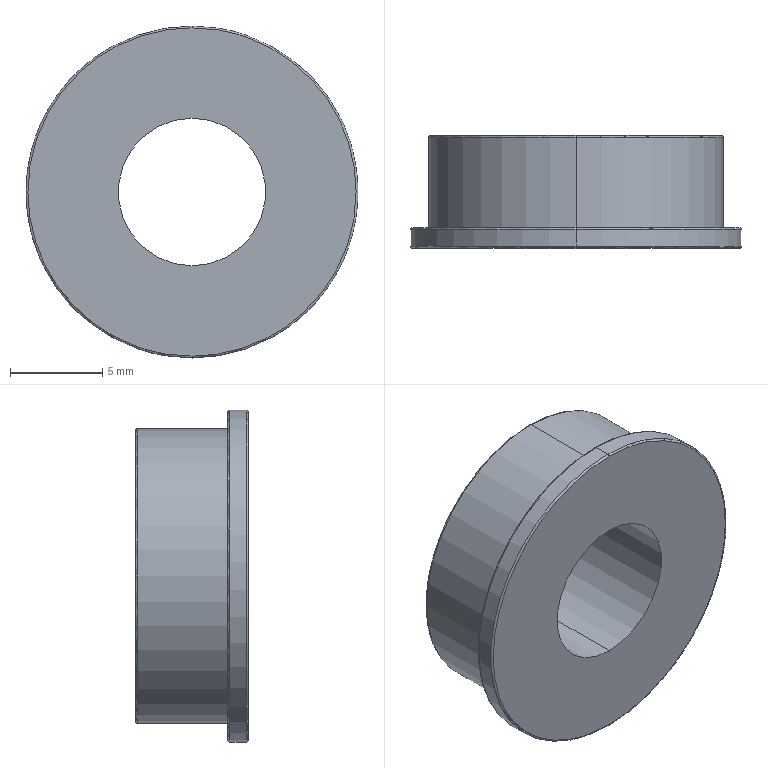Part | NX | features BREP 1 | 1 solid | 15 faces | box 18 x 6.1 x 18 mm | volume 978.51 mm3 | torus 6 | cylinder 6 | plane 3 | commonest cylinder face diameters 8 x2 16 x2 18 x2
STEP:
#1=CARTESIAN_POINT('',(0.,0.,8.9));
#2=VERTEX_POINT('',#1);
#3=CARTESIAN_POINT('',(0.,0.,-8.9));
#4=VERTEX_POINT('',#3);
#5=CARTESIAN_POINT('',(0.,0.,8.9));
#6=CARTESIAN_POINT('',(-0.2723,0.,8.9));
#7=CARTESIAN_POINT('',(-0.6789,0.,8.881));
#8=CARTESIAN_POINT('',(-1.15,0.,8.827));
#9=CARTESIAN_POINT('',(-1.385,0.,8.792));
#10=CARTESIAN_POINT('',(-1.486,0.,8.775));
#11=CARTESIAN_POINT('',(-1.553,0.,8.764));
#12=CARTESIAN_POINT('',(-1.584,0.,8.758));
#13=CARTESIAN_POINT('',(-1.903,0.,8.699));
#14=CARTESIAN_POINT('',(-2.323,0.,8.6));
#15=CARTESIAN_POINT('',(-2.803,0.,8.449));
#16=CARTESIAN_POINT('',(-3.04,0.,8.365));
#17=CARTESIAN_POINT('',(-3.141,0.,8.327));
#18=CARTESIAN_POINT('',(-3.209,0.,8.301));
#19=CARTESIAN_POINT('',(-3.241,0.,8.289));
#20=CARTESIAN_POINT('',(-3.556,0.,8.164));
#21=CARTESIAN_POINT('',(-3.964,0.,7.978));
#22=CARTESIAN_POINT('',(-4.423,0.,7.726));
#23=CARTESIAN_POINT('',(-4.616,0.,7.61));
#24=CARTESIAN_POINT('',(-4.744,0.,7.531));
#25=CARTESIAN_POINT('',(-4.806,0.,7.491));
#26=CARTESIAN_POINT('',(-5.384,0.,7.113));
#27=CARTESIAN_POINT('',(-5.859,0.,6.727));
#28=CARTESIAN_POINT('',(-6.51,0.,6.076));
#29=CARTESIAN_POINT('',(-6.818,0.,5.735));
#30=CARTESIAN_POINT('',(-7.144,0.,5.312));
#31=CARTESIAN_POINT('',(-7.277,0.,5.124));
#32=CARTESIAN_POINT('',(-7.364,0.,4.998));
#33=CARTESIAN_POINT('',(-7.408,0.,4.933));
#34=CARTESIAN_POINT('',(-7.614,0.,4.619));
#35=CARTESIAN_POINT('',(-7.84,0.,4.231));
#36=CARTESIAN_POINT('',(-8.069,0.,3.76));
#37=CARTESIAN_POINT('',(-8.175,0.,3.519));
#38=CARTESIAN_POINT('',(-8.219,0.,3.415));
#39=CARTESIAN_POINT('',(-8.247,0.,3.346));
#40=CARTESIAN_POINT('',(-8.262,0.,3.31));
#41=CARTESIAN_POINT('',(-8.381,0.,3.008));
#42=CARTESIAN_POINT('',(-8.52,0.,2.6));
#43=CARTESIAN_POINT('',(-8.648,0.,2.113));
#44=CARTESIAN_POINT('',(-8.702,0.,1.867));
#45=CARTESIAN_POINT('',(-8.724,0.,1.761));
#46=CARTESIAN_POINT('',(-8.738,0.,1.69));
#47=CARTESIAN_POINT('',(-8.745,0.,1.653));
#48=CARTESIAN_POINT('',(-8.85,0.,1.085));
#49=CARTESIAN_POINT('',(-8.9,0.,0.544));
#50=CARTESIAN_POINT('',(-8.9,0.,-0.272));
#51=CARTESIAN_POINT('',(-8.881,0.,-0.6784));
#52=CARTESIAN_POINT('',(-8.827,0.,-1.15));
#53=CARTESIAN_POINT('',(-8.792,0.,-1.385));
#54=CARTESIAN_POINT('',(-8.775,0.,-1.485));
#55=CARTESIAN_POINT('',(-8.764,0.,-1.553));
#56=CARTESIAN_POINT('',(-8.758,0.,-1.584));
#57=CARTESIAN_POINT('',(-8.699,0.,-1.903));
#58=CARTESIAN_POINT('',(-8.6,0.,-2.323));
#59=CARTESIAN_POINT('',(-8.449,0.,-2.803));
#60=CARTESIAN_POINT('',(-8.365,0.,-3.04));
#61=CARTESIAN_POINT('',(-8.327,0.,-3.141));
#62=CARTESIAN_POINT('',(-8.301,0.,-3.209));
#63=CARTESIAN_POINT('',(-8.289,0.,-3.241));
#64=CARTESIAN_POINT('',(-8.164,0.,-3.556));
#65=CARTESIAN_POINT('',(-7.978,0.,-3.964));
#66=CARTESIAN_POINT('',(-7.726,0.,-4.423));
#67=CARTESIAN_POINT('',(-7.61,0.,-4.616));
#68=CARTESIAN_POINT('',(-7.531,0.,-4.744));
#69=CARTESIAN_POINT('',(-7.491,0.,-4.806));
#70=CARTESIAN_POINT('',(-7.113,0.,-5.384));
#71=CARTESIAN_POINT('',(-6.727,0.,-5.859));
#72=CARTESIAN_POINT('',(-6.076,0.,-6.51));
#73=CARTESIAN_POINT('',(-5.735,0.,-6.818));
#74=CARTESIAN_POINT('',(-5.312,0.,-7.144));
#75=CARTESIAN_POINT('',(-5.124,0.,-7.277));
#76=CARTESIAN_POINT('',(-4.998,0.,-7.364));
#77=CARTESIAN_POINT('',(-4.933,0.,-7.408));
#78=CARTESIAN_POINT('',(-4.619,0.,-7.614));
#79=CARTESIAN_POINT('',(-4.231,0.,-7.84));
#80=CARTESIAN_POINT('',(-3.76,0.,-8.069));
#81=CARTESIAN_POINT('',(-3.519,0.,-8.175));
#82=CARTESIAN_POINT('',(-3.415,0.,-8.219));
#83=CARTESIAN_POINT('',(-3.346,0.,-8.247));
#84=CARTESIAN_POINT('',(-3.31,0.,-8.262));
#85=CARTESIAN_POINT('',(-3.008,0.,-8.381));
#86=CARTESIAN_POINT('',(-2.6,0.,-8.52));
#87=CARTESIAN_POINT('',(-2.113,0.,-8.648));
#88=CARTESIAN_POINT('',(-1.867,0.,-8.702));
#89=CARTESIAN_POINT('',(-1.761,0.,-8.724));
#90=CARTESIAN_POINT('',(-1.69,0.,-8.738));
#91=CARTESIAN_POINT('',(-1.653,0.,-8.745));
#92=CARTESIAN_POINT('',(-1.085,0.,-8.85));
#93=CARTESIAN_POINT('',(-0.5449,0.,-8.9));
#94=CARTESIAN_POINT('',(0.,0.,-8.9));
#95=B_SPLINE_CURVE_WITH_KNOTS('',3,(#5,#6,#7,#8,#9,#10,#11,#12,#13,#14,#15,#16,#17,#18,#19,#20,#21,#22,#23,#24,#25,#26,#27,#28,#29,#30,#31,#32,#33,#34,#35,#36,#37,#38,#39,#40,#41,#42,#43,#44,#45,#46,#47,#48,#49,#50,#51,#52,#53,#54,#55,#56,#57,#58,#59,#60,#61,#62,#63,#64,#65,#66,#67,#68,#69,#70,#71,#72,#73,#74,#75,#76,#77,#78,#79,#80,#81,#82,#83,#84,#85,#86,#87,#88,#89,#90,#91,#92,#93,#94),.UNSPECIFIED.,.F.,.F.,(4,1,1,1,2,2,1,1,1,2,2,1,1,2,2,2,1,1,2,2,1,1,1,2,2,1,1,1,2,2,2,1,1,1,2,2,1,1,1,2,2,1,1,2,2,2,1,1,2,2,1,1,1,2,2,1,1,1,2,2,4),(0.,0.03125,0.04688,0.05469,0.05859,0.0625,0.09375,0.1094,0.1172,0.1211,0.125,0.1562,0.1719,0.1797,0.1875,0.25,0.2812,0.2969,0.3047,0.3125,0.3438,0.3594,0.3672,0.3711,0.375,0.4062,0.4219,0.4297,0.4336,0.4375,0.5,0.5312,0.5469,0.5547,0.5586,0.5625,0.5938,0.6094,0.6172,0.6211,0.625,0.6562,0.6719,0.6797,0.6875,0.75,0.7812,0.7969,0.8047,0.8125,0.8438,0.8594,0.8672,0.8711,0.875,0.9062,0.9219,0.9297,0.9336,0.9375,1.),.UNSPECIFIED.);
#96=EDGE_CURVE('',#2,#4,#95,.T.);
#97=ORIENTED_EDGE('',*,*,#96,.F.);
#98=CARTESIAN_POINT('',(0.,0.1,9.));
#99=VERTEX_POINT('',#98);
#100=CARTESIAN_POINT('',(0.,0.1,8.9));
#101=DIRECTION('',(-1.,0.,0.));
#102=DIRECTION('',(0.,0.,1.));
#103=AXIS2_PLACEMENT_3D('',#100,#101,#102);
#104=CIRCLE('',#103,0.1);
#105=EDGE_CURVE('',#2,#99,#104,.T.);
#106=ORIENTED_EDGE('',*,*,#105,.T.);
#107=CARTESIAN_POINT('',(0.,0.1,-9.));
#108=VERTEX_POINT('',#107);
#109=CARTESIAN_POINT('',(0.,0.1,0.));
#110=DIRECTION('',(0.,-1.,0.));
#111=DIRECTION('',(0.,0.,-1.));
#112=AXIS2_PLACEMENT_3D('',#109,#110,#111);
#113=CIRCLE('',#112,9.);
#114=EDGE_CURVE('',#99,#108,#113,.T.);
#115=ORIENTED_EDGE('',*,*,#114,.T.);
#116=CARTESIAN_POINT('',(0.,0.1,-8.9));
#117=DIRECTION('',(1.,0.,0.));
#118=DIRECTION('',(0.,0.,-1.));
#119=AXIS2_PLACEMENT_3D('',#116,#117,#118);
#120=CIRCLE('',#119,0.1);
#121=EDGE_CURVE('',#4,#108,#120,.T.);
#122=ORIENTED_EDGE('',*,*,#121,.F.);
#123=EDGE_LOOP('',(#97,#106,#115,#122));
#124=FACE_BOUND('',#123,.T.);
#125=CARTESIAN_POINT('',(0.,0.1,0.));
#126=DIRECTION('',(0.,1.,0.));
#127=DIRECTION('',(-1.,0.,0.));
#128=AXIS2_PLACEMENT_3D('',#125,#126,#127);
#129=TOROIDAL_SURFACE('',#128,8.9,0.1);
#130=ADVANCED_FACE('',(#124),#129,.T.);
#131=CARTESIAN_POINT('',(0.,6.,-8.));
#132=VERTEX_POINT('',#131);
#133=CARTESIAN_POINT('',(0.,6.,8.));
#134=VERTEX_POINT('',#133);
#135=CARTESIAN_POINT('',(0.,6.,0.));
#136=DIRECTION('',(0.,1.,0.));
#137=DIRECTION('',(0.,0.,-1.));
#138=AXIS2_PLACEMENT_3D('',#135,#136,#137);
#139=CIRCLE('',#138,8.);
#140=EDGE_CURVE('',#132,#134,#139,.T.);
#141=ORIENTED_EDGE('',*,*,#140,.T.);
#142=CARTESIAN_POINT('',(0.,6.1,7.9));
#143=VERTEX_POINT('',#142);
#144=CARTESIAN_POINT('',(0.,6.,7.9));
#145=DIRECTION('',(-1.,0.,0.));
#146=DIRECTION('',(0.,0.,1.));
#147=AXIS2_PLACEMENT_3D('',#144,#145,#146);
#148=CIRCLE('',#147,0.1);
#149=EDGE_CURVE('',#134,#143,#148,.T.);
#150=ORIENTED_EDGE('',*,*,#149,.T.);
#151=CARTESIAN_POINT('',(0.,6.1,-7.9));
#152=VERTEX_POINT('',#151);
#153=CARTESIAN_POINT('',(0.,6.1,-7.9));
#154=CARTESIAN_POINT('',(-0.2417,6.1,-7.9));
#155=CARTESIAN_POINT('',(-0.6026,6.1,-7.883));
#156=CARTESIAN_POINT('',(-1.021,6.1,-7.835));
#157=CARTESIAN_POINT('',(-1.229,6.1,-7.804));
#158=CARTESIAN_POINT('',(-1.319,6.1,-7.789));
#159=CARTESIAN_POINT('',(-1.378,6.1,-7.779));
#160=CARTESIAN_POINT('',(-1.406,6.1,-7.774));
#161=CARTESIAN_POINT('',(-1.689,6.1,-7.722));
#162=CARTESIAN_POINT('',(-2.062,6.1,-7.634));
#163=CARTESIAN_POINT('',(-2.488,6.1,-7.5));
#164=CARTESIAN_POINT('',(-2.699,6.1,-7.425));
#165=CARTESIAN_POINT('',(-2.788,6.1,-7.392));
#166=CARTESIAN_POINT('',(-2.848,6.1,-7.369));
#167=CARTESIAN_POINT('',(-2.877,6.1,-7.358));
#168=CARTESIAN_POINT('',(-3.156,6.1,-7.247));
#169=CARTESIAN_POINT('',(-3.519,6.1,-7.082));
#170=CARTESIAN_POINT('',(-3.926,6.1,-6.858));
#171=CARTESIAN_POINT('',(-4.097,6.1,-6.755));
#172=CARTESIAN_POINT('',(-4.211,6.1,-6.685));
#173=CARTESIAN_POINT('',(-4.266,6.1,-6.65));
#174=CARTESIAN_POINT('',(-4.779,6.1,-6.314));
#175=CARTESIAN_POINT('',(-5.201,6.1,-5.972));
#176=CARTESIAN_POINT('',(-5.779,6.1,-5.393));
#177=CARTESIAN_POINT('',(-6.052,6.1,-5.091));
#178=CARTESIAN_POINT('',(-6.341,6.1,-4.715));
#179=CARTESIAN_POINT('',(-6.46,6.1,-4.549));
#180=CARTESIAN_POINT('',(-6.537,6.1,-4.437));
#181=CARTESIAN_POINT('',(-6.576,6.1,-4.379));
#182=CARTESIAN_POINT('',(-6.758,6.1,-4.1));
#183=CARTESIAN_POINT('',(-6.959,6.1,-3.755));
#184=CARTESIAN_POINT('',(-7.163,6.1,-3.337));
#185=CARTESIAN_POINT('',(-7.257,6.1,-3.124));
#186=CARTESIAN_POINT('',(-7.295,6.1,-3.032));
#187=CARTESIAN_POINT('',(-7.321,6.1,-2.97));
#188=CARTESIAN_POINT('',(-7.334,6.1,-2.938));
#189=CARTESIAN_POINT('',(-7.44,6.1,-2.67));
#190=CARTESIAN_POINT('',(-7.563,6.1,-2.308));
#191=CARTESIAN_POINT('',(-7.676,6.1,-1.876));
#192=CARTESIAN_POINT('',(-7.725,6.1,-1.657));
#193=CARTESIAN_POINT('',(-7.744,6.1,-1.563));
#194=CARTESIAN_POINT('',(-7.756,6.1,-1.5));
#195=CARTESIAN_POINT('',(-7.763,6.1,-1.467));
#196=CARTESIAN_POINT('',(-7.856,6.1,-0.9627));
#197=CARTESIAN_POINT('',(-7.9,6.1,-0.4828));
#198=CARTESIAN_POINT('',(-7.9,6.1,0.2414));
#199=CARTESIAN_POINT('',(-7.884,6.1,0.6022));
#200=CARTESIAN_POINT('',(-7.835,6.1,1.021));
#201=CARTESIAN_POINT('',(-7.804,6.1,1.229));
#202=CARTESIAN_POINT('',(-7.789,6.1,1.319));
#203=CARTESIAN_POINT('',(-7.779,6.1,1.378));
#204=CARTESIAN_POINT('',(-7.774,6.1,1.406));
#205=CARTESIAN_POINT('',(-7.722,6.1,1.689));
#206=CARTESIAN_POINT('',(-7.634,6.1,2.062));
#207=CARTESIAN_POINT('',(-7.5,6.1,2.488));
#208=CARTESIAN_POINT('',(-7.425,6.1,2.699));
#209=CARTESIAN_POINT('',(-7.392,6.1,2.788));
#210=CARTESIAN_POINT('',(-7.369,6.1,2.848));
#211=CARTESIAN_POINT('',(-7.358,6.1,2.877));
#212=CARTESIAN_POINT('',(-7.247,6.1,3.156));
#213=CARTESIAN_POINT('',(-7.082,6.1,3.519));
#214=CARTESIAN_POINT('',(-6.858,6.1,3.926));
#215=CARTESIAN_POINT('',(-6.755,6.1,4.097));
#216=CARTESIAN_POINT('',(-6.685,6.1,4.211));
#217=CARTESIAN_POINT('',(-6.65,6.1,4.266));
#218=CARTESIAN_POINT('',(-6.314,6.1,4.779));
#219=CARTESIAN_POINT('',(-5.972,6.1,5.201));
#220=CARTESIAN_POINT('',(-5.393,6.1,5.779));
#221=CARTESIAN_POINT('',(-5.091,6.1,6.052));
#222=CARTESIAN_POINT('',(-4.715,6.1,6.341));
#223=CARTESIAN_POINT('',(-4.549,6.1,6.46));
#224=CARTESIAN_POINT('',(-4.437,6.1,6.537));
#225=CARTESIAN_POINT('',(-4.379,6.1,6.576));
#226=CARTESIAN_POINT('',(-4.1,6.1,6.758));
#227=CARTESIAN_POINT('',(-3.755,6.1,6.959));
#228=CARTESIAN_POINT('',(-3.337,6.1,7.163));
#229=CARTESIAN_POINT('',(-3.124,6.1,7.257));
#230=CARTESIAN_POINT('',(-3.032,6.1,7.295));
#231=CARTESIAN_POINT('',(-2.97,6.1,7.321));
#232=CARTESIAN_POINT('',(-2.938,6.1,7.334));
#233=CARTESIAN_POINT('',(-2.67,6.1,7.44));
#234=CARTESIAN_POINT('',(-2.308,6.1,7.563));
#235=CARTESIAN_POINT('',(-1.876,6.1,7.676));
#236=CARTESIAN_POINT('',(-1.657,6.1,7.725));
#237=CARTESIAN_POINT('',(-1.563,6.1,7.744));
#238=CARTESIAN_POINT('',(-1.5,6.1,7.756));
#239=CARTESIAN_POINT('',(-1.467,6.1,7.763));
#240=CARTESIAN_POINT('',(-0.9629,6.1,7.856));
#241=CARTESIAN_POINT('',(-0.4837,6.1,7.9));
#242=CARTESIAN_POINT('',(0.,6.1,7.9));
#243=B_SPLINE_CURVE_WITH_KNOTS('',3,(#153,#154,#155,#156,#157,#158,#159,#160,#161,#162,#163,#164,#165,#166,#167,#168,#169,#170,#171,#172,#173,#174,#175,#176,#177,#178,#179,#180,#181,#182,#183,#184,#185,#186,#187,#188,#189,#190,#191,#192,#193,#194,#195,#196,#197,#198,#199,#200,#201,#202,#203,#204,#205,#206,#207,#208,#209,#210,#211,#212,#213,#214,#215,#216,#217,#218,#219,#220,#221,#222,#223,#224,#225,#226,#227,#228,#229,#230,#231,#232,#233,#234,#235,#236,#237,#238,#239,#240,#241,#242),.UNSPECIFIED.,.F.,.F.,(4,1,1,1,2,2,1,1,1,2,2,1,1,2,2,2,1,1,2,2,1,1,1,2,2,1,1,1,2,2,2,1,1,1,2,2,1,1,1,2,2,1,1,2,2,2,1,1,2,2,1,1,1,2,2,1,1,1,2,2,4),(0.,0.03125,0.04688,0.05469,0.05859,0.0625,0.09375,0.1094,0.1172,0.1211,0.125,0.1562,0.1719,0.1797,0.1875,0.25,0.2812,0.2969,0.3047,0.3125,0.3438,0.3594,0.3672,0.3711,0.375,0.4062,0.4219,0.4297,0.4336,0.4375,0.5,0.5312,0.5469,0.5547,0.5586,0.5625,0.5938,0.6094,0.6172,0.6211,0.625,0.6562,0.6719,0.6797,0.6875,0.75,0.7812,0.7969,0.8047,0.8125,0.8438,0.8594,0.8672,0.8711,0.875,0.9062,0.9219,0.9297,0.9336,0.9375,1.),.UNSPECIFIED.);
#244=EDGE_CURVE('',#152,#143,#243,.T.);
#245=ORIENTED_EDGE('',*,*,#244,.F.);
#246=CARTESIAN_POINT('',(0.,6.,-7.9));
#247=DIRECTION('',(1.,0.,0.));
#248=DIRECTION('',(0.,0.,-1.));
#249=AXIS2_PLACEMENT_3D('',#246,#247,#248);
#250=CIRCLE('',#249,0.1);
#251=EDGE_CURVE('',#132,#152,#250,.T.);
#252=ORIENTED_EDGE('',*,*,#251,.F.);
#253=EDGE_LOOP('',(#141,#150,#245,#252));
#254=FACE_BOUND('',#253,.T.);
#255=CARTESIAN_POINT('',(0.,6.,0.));
#256=DIRECTION('',(0.,1.,0.));
#257=DIRECTION('',(-1.,0.,0.));
#258=AXIS2_PLACEMENT_3D('',#255,#256,#257);
#259=TOROIDAL_SURFACE('',#258,7.9,0.1);
#260=ADVANCED_FACE('',(#254),#259,.T.);
#261=CARTESIAN_POINT('',(0.,1.,9.));
#262=VERTEX_POINT('',#261);
#263=CARTESIAN_POINT('',(0.,1.,-9.));
#264=VERTEX_POINT('',#263);
#265=CARTESIAN_POINT('',(0.,1.,0.));
#266=DIRECTION('',(0.,-1.,0.));
#267=DIRECTION('',(0.,0.,-1.));
#268=AXIS2_PLACEMENT_3D('',#265,#266,#267);
#269=CIRCLE('',#268,9.);
#270=EDGE_CURVE('',#262,#264,#269,.T.);
#271=ORIENTED_EDGE('',*,*,#270,.F.);
#272=CARTESIAN_POINT('',(0.,1.1,8.9));
#273=VERTEX_POINT('',#272);
#274=CARTESIAN_POINT('',(0.,1.,8.9));
#275=DIRECTION('',(-1.,0.,0.));
#276=DIRECTION('',(0.,0.,1.));
#277=AXIS2_PLACEMENT_3D('',#274,#275,#276);
#278=CIRCLE('',#277,0.1);
#279=EDGE_CURVE('',#262,#273,#278,.T.);
#280=ORIENTED_EDGE('',*,*,#279,.T.);
#281=CARTESIAN_POINT('',(0.,1.1,-8.9));
#282=VERTEX_POINT('',#281);
#283=CARTESIAN_POINT('',(0.,1.1,8.9));
#284=CARTESIAN_POINT('',(-17.8,1.1,8.9));
#285=CARTESIAN_POINT('',(-17.8,1.1,-8.9));
#286=CARTESIAN_POINT('',(0.,1.1,-8.9));
#287=(BOUNDED_CURVE()B_SPLINE_CURVE(3,(#283,#284,#285,#286),.UNSPECIFIED.,.F.,.F.)B_SPLINE_CURVE_WITH_KNOTS((4,4),(0.,1.),.UNSPECIFIED.)CURVE()GEOMETRIC_REPRESENTATION_ITEM()RATIONAL_B_SPLINE_CURVE((1.,0.3333,0.3333,1.))REPRESENTATION_ITEM(''));
#288=EDGE_CURVE('',#273,#282,#287,.T.);
#289=ORIENTED_EDGE('',*,*,#288,.T.);
#290=CARTESIAN_POINT('',(0.,1.,-8.9));
#291=DIRECTION('',(1.,0.,0.));
#292=DIRECTION('',(0.,0.,-1.));
#293=AXIS2_PLACEMENT_3D('',#290,#291,#292);
#294=CIRCLE('',#293,0.1);
#295=EDGE_CURVE('',#264,#282,#294,.T.);
#296=ORIENTED_EDGE('',*,*,#295,.F.);
#297=EDGE_LOOP('',(#271,#280,#289,#296));
#298=FACE_BOUND('',#297,.T.);
#299=CARTESIAN_POINT('',(0.,1.,0.));
#300=DIRECTION('',(0.,1.,0.));
#301=DIRECTION('',(-1.,0.,0.));
#302=AXIS2_PLACEMENT_3D('',#299,#300,#301);
#303=TOROIDAL_SURFACE('',#302,8.9,0.1);
#304=ADVANCED_FACE('',(#298),#303,.T.);
#305=CARTESIAN_POINT('',(0.,6.1,4.));
#306=VERTEX_POINT('',#305);
#307=CARTESIAN_POINT('',(0.,6.1,-4.));
#308=VERTEX_POINT('',#307);
#309=CARTESIAN_POINT('',(0.,6.1,0.));
#310=DIRECTION('',(0.,-1.,0.));
#311=DIRECTION('',(0.,0.,-1.));
#312=AXIS2_PLACEMENT_3D('',#309,#310,#311);
#313=CIRCLE('',#312,4.);
#314=EDGE_CURVE('',#306,#308,#313,.T.);
#315=ORIENTED_EDGE('',*,*,#314,.F.);
#316=CARTESIAN_POINT('',(0.,0.,4.));
#317=VERTEX_POINT('',#316);
#318=CARTESIAN_POINT('',(0.,0.,4.));
#319=DIRECTION('',(0.,-1.,0.));
#320=VECTOR('',#319,1000.);
#321=LINE('',#318,#320);
#322=EDGE_CURVE('',#306,#317,#321,.T.);
#323=ORIENTED_EDGE('',*,*,#322,.T.);
#324=CARTESIAN_POINT('',(0.,0.,-4.));
#325=VERTEX_POINT('',#324);
#326=CARTESIAN_POINT('',(0.,0.,0.));
#327=DIRECTION('',(0.,1.,0.));
#328=DIRECTION('',(0.,0.,-1.));
#329=AXIS2_PLACEMENT_3D('',#326,#327,#328);
#330=CIRCLE('',#329,4.);
#331=EDGE_CURVE('',#325,#317,#330,.T.);
#332=ORIENTED_EDGE('',*,*,#331,.F.);
#333=CARTESIAN_POINT('',(0.,0.,-4.));
#334=DIRECTION('',(0.,-1.,0.));
#335=VECTOR('',#334,1000.);
#336=LINE('',#333,#335);
#337=EDGE_CURVE('',#308,#325,#336,.T.);
#338=ORIENTED_EDGE('',*,*,#337,.F.);
#339=EDGE_LOOP('',(#315,#323,#332,#338));
#340=FACE_BOUND('',#339,.T.);
#341=CARTESIAN_POINT('',(0.,0.,0.));
#342=DIRECTION('',(0.,-1.,0.));
#343=DIRECTION('',(0.,0.,-1.));
#344=AXIS2_PLACEMENT_3D('',#341,#342,#343);
#345=CYLINDRICAL_SURFACE('',#344,4.);
#346=ADVANCED_FACE('',(#340),#345,.F.);
#347=CARTESIAN_POINT('',(0.,1.,0.));
#348=DIRECTION('',(0.,-1.,0.));
#349=DIRECTION('',(0.,0.,-1.));
#350=AXIS2_PLACEMENT_3D('',#347,#348,#349);
#351=CIRCLE('',#350,9.);
#352=EDGE_CURVE('',#264,#262,#351,.T.);
#353=ORIENTED_EDGE('',*,*,#352,.T.);
#354=CARTESIAN_POINT('',(0.,0.,9.));
#355=DIRECTION('',(0.,-1.,0.));
#356=VECTOR('',#355,1000.);
#357=LINE('',#354,#356);
#358=EDGE_CURVE('',#262,#99,#357,.T.);
#359=ORIENTED_EDGE('',*,*,#358,.T.);
#360=CARTESIAN_POINT('',(0.,0.1,0.));
#361=DIRECTION('',(0.,-1.,0.));
#362=DIRECTION('',(0.,0.,-1.));
#363=AXIS2_PLACEMENT_3D('',#360,#361,#362);
#364=CIRCLE('',#363,9.);
#365=EDGE_CURVE('',#108,#99,#364,.T.);
#366=ORIENTED_EDGE('',*,*,#365,.F.);
#367=CARTESIAN_POINT('',(0.,0.,-9.));
#368=DIRECTION('',(0.,-1.,0.));
#369=VECTOR('',#368,1000.);
#370=LINE('',#367,#369);
#371=EDGE_CURVE('',#264,#108,#370,.T.);
#372=ORIENTED_EDGE('',*,*,#371,.F.);
#373=EDGE_LOOP('',(#353,#359,#366,#372));
#374=FACE_BOUND('',#373,.T.);
#375=CARTESIAN_POINT('',(0.,0.,0.));
#376=DIRECTION('',(0.,-1.,0.));
#377=DIRECTION('',(0.,0.,-1.));
#378=AXIS2_PLACEMENT_3D('',#375,#376,#377);
#379=CYLINDRICAL_SURFACE('',#378,9.);
#380=ADVANCED_FACE('',(#374),#379,.T.);
#381=CARTESIAN_POINT('',(0.,6.,0.));
#382=DIRECTION('',(0.,1.,0.));
#383=DIRECTION('',(0.,0.,-1.));
#384=AXIS2_PLACEMENT_3D('',#381,#382,#383);
#385=CIRCLE('',#384,8.);
#386=EDGE_CURVE('',#134,#132,#385,.T.);
#387=ORIENTED_EDGE('',*,*,#386,.F.);
#388=CARTESIAN_POINT('',(0.,1.1,8.));
#389=VERTEX_POINT('',#388);
#390=CARTESIAN_POINT('',(0.,0.,8.));
#391=DIRECTION('',(0.,-1.,0.));
#392=VECTOR('',#391,1000.);
#393=LINE('',#390,#392);
#394=EDGE_CURVE('',#134,#389,#393,.T.);
#395=ORIENTED_EDGE('',*,*,#394,.T.);
#396=CARTESIAN_POINT('',(0.,1.1,-8.));
#397=VERTEX_POINT('',#396);
#398=CARTESIAN_POINT('',(0.,1.1,0.));
#399=DIRECTION('',(0.,1.,0.));
#400=DIRECTION('',(0.,0.,-1.));
#401=AXIS2_PLACEMENT_3D('',#398,#399,#400);
#402=CIRCLE('',#401,8.);
#403=EDGE_CURVE('',#389,#397,#402,.T.);
#404=ORIENTED_EDGE('',*,*,#403,.T.);
#405=CARTESIAN_POINT('',(0.,0.,-8.));
#406=DIRECTION('',(0.,-1.,0.));
#407=VECTOR('',#406,1000.);
#408=LINE('',#405,#407);
#409=EDGE_CURVE('',#132,#397,#408,.T.);
#410=ORIENTED_EDGE('',*,*,#409,.F.);
#411=EDGE_LOOP('',(#387,#395,#404,#410));
#412=FACE_BOUND('',#411,.T.);
#413=CARTESIAN_POINT('',(0.,0.,0.));
#414=DIRECTION('',(0.,-1.,0.));
#415=DIRECTION('',(0.,0.,-1.));
#416=AXIS2_PLACEMENT_3D('',#413,#414,#415);
#417=CYLINDRICAL_SURFACE('',#416,8.);
#418=ADVANCED_FACE('',(#412),#417,.T.);
#419=CARTESIAN_POINT('',(0.,0.,-8.9));
#420=CARTESIAN_POINT('',(0.2723,0.,-8.9));
#421=CARTESIAN_POINT('',(0.6789,0.,-8.881));
#422=CARTESIAN_POINT('',(1.15,0.,-8.827));
#423=CARTESIAN_POINT('',(1.385,0.,-8.792));
#424=CARTESIAN_POINT('',(1.486,0.,-8.775));
#425=CARTESIAN_POINT('',(1.553,0.,-8.764));
#426=CARTESIAN_POINT('',(1.584,0.,-8.758));
#427=CARTESIAN_POINT('',(1.903,0.,-8.699));
#428=CARTESIAN_POINT('',(2.323,0.,-8.6));
#429=CARTESIAN_POINT('',(2.803,0.,-8.449));
#430=CARTESIAN_POINT('',(3.04,0.,-8.365));
#431=CARTESIAN_POINT('',(3.141,0.,-8.327));
#432=CARTESIAN_POINT('',(3.209,0.,-8.301));
#433=CARTESIAN_POINT('',(3.241,0.,-8.289));
#434=CARTESIAN_POINT('',(3.556,0.,-8.164));
#435=CARTESIAN_POINT('',(3.964,0.,-7.978));
#436=CARTESIAN_POINT('',(4.423,0.,-7.726));
#437=CARTESIAN_POINT('',(4.616,0.,-7.61));
#438=CARTESIAN_POINT('',(4.744,0.,-7.531));
#439=CARTESIAN_POINT('',(4.806,0.,-7.491));
#440=CARTESIAN_POINT('',(5.384,0.,-7.113));
#441=CARTESIAN_POINT('',(5.859,0.,-6.727));
#442=CARTESIAN_POINT('',(6.51,0.,-6.076));
#443=CARTESIAN_POINT('',(6.818,0.,-5.735));
#444=CARTESIAN_POINT('',(7.144,0.,-5.312));
#445=CARTESIAN_POINT('',(7.277,0.,-5.124));
#446=CARTESIAN_POINT('',(7.364,0.,-4.998));
#447=CARTESIAN_POINT('',(7.408,0.,-4.933));
#448=CARTESIAN_POINT('',(7.614,0.,-4.619));
#449=CARTESIAN_POINT('',(7.84,0.,-4.231));
#450=CARTESIAN_POINT('',(8.069,0.,-3.76));
#451=CARTESIAN_POINT('',(8.175,0.,-3.519));
#452=CARTESIAN_POINT('',(8.219,0.,-3.415));
#453=CARTESIAN_POINT('',(8.247,0.,-3.346));
#454=CARTESIAN_POINT('',(8.262,0.,-3.31));
#455=CARTESIAN_POINT('',(8.381,0.,-3.008));
#456=CARTESIAN_POINT('',(8.52,0.,-2.6));
#457=CARTESIAN_POINT('',(8.648,0.,-2.113));
#458=CARTESIAN_POINT('',(8.702,0.,-1.867));
#459=CARTESIAN_POINT('',(8.724,0.,-1.761));
#460=CARTESIAN_POINT('',(8.738,0.,-1.69));
#461=CARTESIAN_POINT('',(8.745,0.,-1.653));
#462=CARTESIAN_POINT('',(8.85,0.,-1.085));
#463=CARTESIAN_POINT('',(8.9,0.,-0.544));
#464=CARTESIAN_POINT('',(8.9,0.,0.272));
#465=CARTESIAN_POINT('',(8.881,0.,0.6784));
#466=CARTESIAN_POINT('',(8.827,0.,1.15));
#467=CARTESIAN_POINT('',(8.792,0.,1.385));
#468=CARTESIAN_POINT('',(8.775,0.,1.485));
#469=CARTESIAN_POINT('',(8.764,0.,1.553));
#470=CARTESIAN_POINT('',(8.758,0.,1.584));
#471=CARTESIAN_POINT('',(8.699,0.,1.903));
#472=CARTESIAN_POINT('',(8.6,0.,2.323));
#473=CARTESIAN_POINT('',(8.449,0.,2.803));
#474=CARTESIAN_POINT('',(8.365,0.,3.04));
#475=CARTESIAN_POINT('',(8.327,0.,3.141));
#476=CARTESIAN_POINT('',(8.301,0.,3.209));
#477=CARTESIAN_POINT('',(8.289,0.,3.241));
#478=CARTESIAN_POINT('',(8.164,0.,3.556));
#479=CARTESIAN_POINT('',(7.978,0.,3.964));
#480=CARTESIAN_POINT('',(7.726,0.,4.423));
#481=CARTESIAN_POINT('',(7.61,0.,4.616));
#482=CARTESIAN_POINT('',(7.531,0.,4.744));
#483=CARTESIAN_POINT('',(7.491,0.,4.806));
#484=CARTESIAN_POINT('',(7.113,0.,5.384));
#485=CARTESIAN_POINT('',(6.727,0.,5.859));
#486=CARTESIAN_POINT('',(6.076,0.,6.51));
#487=CARTESIAN_POINT('',(5.735,0.,6.818));
#488=CARTESIAN_POINT('',(5.312,0.,7.144));
#489=CARTESIAN_POINT('',(5.124,0.,7.277));
#490=CARTESIAN_POINT('',(4.998,0.,7.364));
#491=CARTESIAN_POINT('',(4.933,0.,7.408));
#492=CARTESIAN_POINT('',(4.619,0.,7.614));
#493=CARTESIAN_POINT('',(4.231,0.,7.84));
#494=CARTESIAN_POINT('',(3.76,0.,8.069));
#495=CARTESIAN_POINT('',(3.519,0.,8.175));
#496=CARTESIAN_POINT('',(3.415,0.,8.219));
#497=CARTESIAN_POINT('',(3.346,0.,8.247));
#498=CARTESIAN_POINT('',(3.31,0.,8.262));
#499=CARTESIAN_POINT('',(3.008,0.,8.381));
#500=CARTESIAN_POINT('',(2.6,0.,8.52));
#501=CARTESIAN_POINT('',(2.113,0.,8.648));
#502=CARTESIAN_POINT('',(1.867,0.,8.702));
#503=CARTESIAN_POINT('',(1.761,0.,8.724));
#504=CARTESIAN_POINT('',(1.69,0.,8.738));
#505=CARTESIAN_POINT('',(1.653,0.,8.745));
#506=CARTESIAN_POINT('',(1.085,0.,8.85));
#507=CARTESIAN_POINT('',(0.5449,0.,8.9));
#508=CARTESIAN_POINT('',(0.,0.,8.9));
#509=B_SPLINE_CURVE_WITH_KNOTS('',3,(#419,#420,#421,#422,#423,#424,#425,#426,#427,#428,#429,#430,#431,#432,#433,#434,#435,#436,#437,#438,#439,#440,#441,#442,#443,#444,#445,#446,#447,#448,#449,#450,#451,#452,#453,#454,#455,#456,#457,#458,#459,#460,#461,#462,#463,#464,#465,#466,#467,#468,#469,#470,#471,#472,#473,#474,#475,#476,#477,#478,#479,#480,#481,#482,#483,#484,#485,#486,#487,#488,#489,#490,#491,#492,#493,#494,#495,#496,#497,#498,#499,#500,#501,#502,#503,#504,#505,#506,#507,#508),.UNSPECIFIED.,.F.,.F.,(4,1,1,1,2,2,1,1,1,2,2,1,1,2,2,2,1,1,2,2,1,1,1,2,2,1,1,1,2,2,2,1,1,1,2,2,1,1,1,2,2,1,1,2,2,2,1,1,2,2,1,1,1,2,2,1,1,1,2,2,4),(0.,0.03125,0.04688,0.05469,0.05859,0.0625,0.09375,0.1094,0.1172,0.1211,0.125,0.1562,0.1719,0.1797,0.1875,0.25,0.2813,0.2969,0.3047,0.3125,0.3438,0.3594,0.3672,0.3711,0.375,0.4062,0.4219,0.4297,0.4336,0.4375,0.5,0.5312,0.5469,0.5547,0.5586,0.5625,0.5938,0.6094,0.6172,0.6211,0.625,0.6562,0.6719,0.6797,0.6875,0.75,0.7812,0.7969,0.8047,0.8125,0.8438,0.8594,0.8672,0.8711,0.875,0.9062,0.9219,0.9297,0.9336,0.9375,1.),.UNSPECIFIED.);
#510=EDGE_CURVE('',#4,#2,#509,.T.);
#511=ORIENTED_EDGE('',*,*,#510,.T.);
#512=ORIENTED_EDGE('',*,*,#96,.T.);
#513=EDGE_LOOP('',(#511,#512));
#514=FACE_BOUND('',#513,.T.);
#515=ORIENTED_EDGE('',*,*,#331,.T.);
#516=CARTESIAN_POINT('',(0.,0.,0.));
#517=DIRECTION('',(0.,1.,0.));
#518=DIRECTION('',(0.,0.,-1.));
#519=AXIS2_PLACEMENT_3D('',#516,#517,#518);
#520=CIRCLE('',#519,4.);
#521=EDGE_CURVE('',#317,#325,#520,.T.);
#522=ORIENTED_EDGE('',*,*,#521,.T.);
#523=EDGE_LOOP('',(#515,#522));
#524=FACE_BOUND('',#523,.T.);
#525=CARTESIAN_POINT('',(4.,0.,0.));
#526=DIRECTION('',(0.,-1.,0.));
#527=DIRECTION('',(0.,0.,-1.));
#528=AXIS2_PLACEMENT_3D('',#525,#526,#527);
#529=PLANE('',#528);
#530=ADVANCED_FACE('',(#514,#524),#529,.T.);
#531=ORIENTED_EDGE('',*,*,#322,.F.);
#532=CARTESIAN_POINT('',(0.,6.1,0.));
#533=DIRECTION('',(0.,-1.,0.));
#534=DIRECTION('',(0.,0.,-1.));
#535=AXIS2_PLACEMENT_3D('',#532,#533,#534);
#536=CIRCLE('',#535,4.);
#537=EDGE_CURVE('',#308,#306,#536,.T.);
#538=ORIENTED_EDGE('',*,*,#537,.F.);
#539=ORIENTED_EDGE('',*,*,#337,.T.);
#540=ORIENTED_EDGE('',*,*,#521,.F.);
#541=EDGE_LOOP('',(#531,#538,#539,#540));
#542=FACE_BOUND('',#541,.T.);
#543=CARTESIAN_POINT('',(0.,0.,0.));
#544=DIRECTION('',(0.,-1.,0.));
#545=DIRECTION('',(0.,0.,-1.));
#546=AXIS2_PLACEMENT_3D('',#543,#544,#545);
#547=CYLINDRICAL_SURFACE('',#546,4.);
#548=ADVANCED_FACE('',(#542),#547,.F.);
#549=ORIENTED_EDGE('',*,*,#105,.F.);
#550=ORIENTED_EDGE('',*,*,#510,.F.);
#551=ORIENTED_EDGE('',*,*,#121,.T.);
#552=ORIENTED_EDGE('',*,*,#365,.T.);
#553=EDGE_LOOP('',(#549,#550,#551,#552));
#554=FACE_BOUND('',#553,.T.);
#555=CARTESIAN_POINT('',(0.,0.1,0.));
#556=DIRECTION('',(0.,1.,0.));
#557=DIRECTION('',(-1.,0.,0.));
#558=AXIS2_PLACEMENT_3D('',#555,#556,#557);
#559=TOROIDAL_SURFACE('',#558,8.9,0.1);
#560=ADVANCED_FACE('',(#554),#559,.T.);
#561=CARTESIAN_POINT('',(0.,6.1,7.9));
#562=CARTESIAN_POINT('',(0.2417,6.1,7.9));
#563=CARTESIAN_POINT('',(0.6026,6.1,7.883));
#564=CARTESIAN_POINT('',(1.021,6.1,7.835));
#565=CARTESIAN_POINT('',(1.229,6.1,7.804));
#566=CARTESIAN_POINT('',(1.319,6.1,7.789));
#567=CARTESIAN_POINT('',(1.378,6.1,7.779));
#568=CARTESIAN_POINT('',(1.406,6.1,7.774));
#569=CARTESIAN_POINT('',(1.689,6.1,7.722));
#570=CARTESIAN_POINT('',(2.062,6.1,7.634));
#571=CARTESIAN_POINT('',(2.488,6.1,7.5));
#572=CARTESIAN_POINT('',(2.699,6.1,7.425));
#573=CARTESIAN_POINT('',(2.788,6.1,7.392));
#574=CARTESIAN_POINT('',(2.848,6.1,7.369));
#575=CARTESIAN_POINT('',(2.877,6.1,7.358));
#576=CARTESIAN_POINT('',(3.156,6.1,7.247));
#577=CARTESIAN_POINT('',(3.519,6.1,7.082));
#578=CARTESIAN_POINT('',(3.926,6.1,6.858));
#579=CARTESIAN_POINT('',(4.097,6.1,6.755));
#580=CARTESIAN_POINT('',(4.211,6.1,6.685));
#581=CARTESIAN_POINT('',(4.266,6.1,6.65));
#582=CARTESIAN_POINT('',(4.779,6.1,6.314));
#583=CARTESIAN_POINT('',(5.201,6.1,5.972));
#584=CARTESIAN_POINT('',(5.779,6.1,5.393));
#585=CARTESIAN_POINT('',(6.052,6.1,5.091));
#586=CARTESIAN_POINT('',(6.341,6.1,4.715));
#587=CARTESIAN_POINT('',(6.46,6.1,4.549));
#588=CARTESIAN_POINT('',(6.537,6.1,4.437));
#589=CARTESIAN_POINT('',(6.576,6.1,4.379));
#590=CARTESIAN_POINT('',(6.758,6.1,4.1));
#591=CARTESIAN_POINT('',(6.959,6.1,3.755));
#592=CARTESIAN_POINT('',(7.163,6.1,3.337));
#593=CARTESIAN_POINT('',(7.257,6.1,3.124));
#594=CARTESIAN_POINT('',(7.295,6.1,3.032));
#595=CARTESIAN_POINT('',(7.321,6.1,2.97));
#596=CARTESIAN_POINT('',(7.334,6.1,2.938));
#597=CARTESIAN_POINT('',(7.44,6.1,2.67));
#598=CARTESIAN_POINT('',(7.563,6.1,2.308));
#599=CARTESIAN_POINT('',(7.676,6.1,1.876));
#600=CARTESIAN_POINT('',(7.725,6.1,1.657));
#601=CARTESIAN_POINT('',(7.744,6.1,1.563));
#602=CARTESIAN_POINT('',(7.756,6.1,1.5));
#603=CARTESIAN_POINT('',(7.763,6.1,1.467));
#604=CARTESIAN_POINT('',(7.856,6.1,0.9627));
#605=CARTESIAN_POINT('',(7.9,6.1,0.4828));
#606=CARTESIAN_POINT('',(7.9,6.1,-0.2414));
#607=CARTESIAN_POINT('',(7.884,6.1,-0.6022));
#608=CARTESIAN_POINT('',(7.835,6.1,-1.021));
#609=CARTESIAN_POINT('',(7.804,6.1,-1.229));
#610=CARTESIAN_POINT('',(7.789,6.1,-1.319));
#611=CARTESIAN_POINT('',(7.779,6.1,-1.378));
#612=CARTESIAN_POINT('',(7.774,6.1,-1.406));
#613=CARTESIAN_POINT('',(7.722,6.1,-1.689));
#614=CARTESIAN_POINT('',(7.634,6.1,-2.062));
#615=CARTESIAN_POINT('',(7.5,6.1,-2.488));
#616=CARTESIAN_POINT('',(7.425,6.1,-2.699));
#617=CARTESIAN_POINT('',(7.392,6.1,-2.788));
#618=CARTESIAN_POINT('',(7.369,6.1,-2.848));
#619=CARTESIAN_POINT('',(7.358,6.1,-2.877));
#620=CARTESIAN_POINT('',(7.247,6.1,-3.156));
#621=CARTESIAN_POINT('',(7.082,6.1,-3.519));
#622=CARTESIAN_POINT('',(6.858,6.1,-3.926));
#623=CARTESIAN_POINT('',(6.755,6.1,-4.097));
#624=CARTESIAN_POINT('',(6.685,6.1,-4.211));
#625=CARTESIAN_POINT('',(6.65,6.1,-4.266));
#626=CARTESIAN_POINT('',(6.314,6.1,-4.779));
#627=CARTESIAN_POINT('',(5.972,6.1,-5.201));
#628=CARTESIAN_POINT('',(5.393,6.1,-5.779));
#629=CARTESIAN_POINT('',(5.091,6.1,-6.052));
#630=CARTESIAN_POINT('',(4.715,6.1,-6.341));
#631=CARTESIAN_POINT('',(4.549,6.1,-6.46));
#632=CARTESIAN_POINT('',(4.437,6.1,-6.537));
#633=CARTESIAN_POINT('',(4.379,6.1,-6.576));
#634=CARTESIAN_POINT('',(4.1,6.1,-6.758));
#635=CARTESIAN_POINT('',(3.755,6.1,-6.959));
#636=CARTESIAN_POINT('',(3.337,6.1,-7.163));
#637=CARTESIAN_POINT('',(3.124,6.1,-7.257));
#638=CARTESIAN_POINT('',(3.032,6.1,-7.295));
#639=CARTESIAN_POINT('',(2.97,6.1,-7.321));
#640=CARTESIAN_POINT('',(2.938,6.1,-7.334));
#641=CARTESIAN_POINT('',(2.67,6.1,-7.44));
#642=CARTESIAN_POINT('',(2.308,6.1,-7.563));
#643=CARTESIAN_POINT('',(1.876,6.1,-7.676));
#644=CARTESIAN_POINT('',(1.657,6.1,-7.725));
#645=CARTESIAN_POINT('',(1.563,6.1,-7.744));
#646=CARTESIAN_POINT('',(1.5,6.1,-7.756));
#647=CARTESIAN_POINT('',(1.467,6.1,-7.763));
#648=CARTESIAN_POINT('',(0.9629,6.1,-7.856));
#649=CARTESIAN_POINT('',(0.4837,6.1,-7.9));
#650=CARTESIAN_POINT('',(0.,6.1,-7.9));
#651=B_SPLINE_CURVE_WITH_KNOTS('',3,(#561,#562,#563,#564,#565,#566,#567,#568,#569,#570,#571,#572,#573,#574,#575,#576,#577,#578,#579,#580,#581,#582,#583,#584,#585,#586,#587,#588,#589,#590,#591,#592,#593,#594,#595,#596,#597,#598,#599,#600,#601,#602,#603,#604,#605,#606,#607,#608,#609,#610,#611,#612,#613,#614,#615,#616,#617,#618,#619,#620,#621,#622,#623,#624,#625,#626,#627,#628,#629,#630,#631,#632,#633,#634,#635,#636,#637,#638,#639,#640,#641,#642,#643,#644,#645,#646,#647,#648,#649,#650),.UNSPECIFIED.,.F.,.F.,(4,1,1,1,2,2,1,1,1,2,2,1,1,2,2,2,1,1,2,2,1,1,1,2,2,1,1,1,2,2,2,1,1,1,2,2,1,1,1,2,2,1,1,2,2,2,1,1,2,2,1,1,1,2,2,1,1,1,2,2,4),(0.,0.03125,0.04688,0.05469,0.05859,0.0625,0.09375,0.1094,0.1172,0.1211,0.125,0.1562,0.1719,0.1797,0.1875,0.25,0.2812,0.2969,0.3047,0.3125,0.3438,0.3594,0.3672,0.3711,0.375,0.4062,0.4219,0.4297,0.4336,0.4375,0.5,0.5312,0.5469,0.5547,0.5586,0.5625,0.5938,0.6094,0.6172,0.6211,0.625,0.6562,0.6719,0.6797,0.6875,0.75,0.7812,0.7969,0.8047,0.8125,0.8438,0.8594,0.8672,0.8711,0.875,0.9062,0.9219,0.9297,0.9336,0.9375,1.),.UNSPECIFIED.);
#652=EDGE_CURVE('',#143,#152,#651,.T.);
#653=ORIENTED_EDGE('',*,*,#652,.T.);
#654=ORIENTED_EDGE('',*,*,#244,.T.);
#655=EDGE_LOOP('',(#653,#654));
#656=FACE_BOUND('',#655,.T.);
#657=ORIENTED_EDGE('',*,*,#537,.T.);
#658=ORIENTED_EDGE('',*,*,#314,.T.);
#659=EDGE_LOOP('',(#657,#658));
#660=FACE_BOUND('',#659,.T.);
#661=CARTESIAN_POINT('',(7.9,6.1,0.));
#662=DIRECTION('',(0.,1.,0.));
#663=DIRECTION('',(1.,0.,0.));
#664=AXIS2_PLACEMENT_3D('',#661,#662,#663);
#665=PLANE('',#664);
#666=ADVANCED_FACE('',(#656,#660),#665,.T.);
#667=ORIENTED_EDGE('',*,*,#358,.F.);
#668=ORIENTED_EDGE('',*,*,#270,.T.);
#669=ORIENTED_EDGE('',*,*,#371,.T.);
#670=ORIENTED_EDGE('',*,*,#114,.F.);
#671=EDGE_LOOP('',(#667,#668,#669,#670));
#672=FACE_BOUND('',#671,.T.);
#673=CARTESIAN_POINT('',(0.,0.,0.));
#674=DIRECTION('',(0.,-1.,0.));
#675=DIRECTION('',(0.,0.,-1.));
#676=AXIS2_PLACEMENT_3D('',#673,#674,#675);
#677=CYLINDRICAL_SURFACE('',#676,9.);
#678=ADVANCED_FACE('',(#672),#677,.T.);
#679=ORIENTED_EDGE('',*,*,#149,.F.);
#680=ORIENTED_EDGE('',*,*,#386,.T.);
#681=ORIENTED_EDGE('',*,*,#251,.T.);
#682=ORIENTED_EDGE('',*,*,#652,.F.);
#683=EDGE_LOOP('',(#679,#680,#681,#682));
#684=FACE_BOUND('',#683,.T.);
#685=CARTESIAN_POINT('',(0.,6.,0.));
#686=DIRECTION('',(0.,1.,0.));
#687=DIRECTION('',(-1.,0.,0.));
#688=AXIS2_PLACEMENT_3D('',#685,#686,#687);
#689=TOROIDAL_SURFACE('',#688,7.9,0.1);
#690=ADVANCED_FACE('',(#684),#689,.T.);
#691=ORIENTED_EDGE('',*,*,#279,.F.);
#692=ORIENTED_EDGE('',*,*,#352,.F.);
#693=ORIENTED_EDGE('',*,*,#295,.T.);
#694=CARTESIAN_POINT('',(0.,1.1,-8.9));
#695=CARTESIAN_POINT('',(17.8,1.1,-8.9));
#696=CARTESIAN_POINT('',(17.8,1.1,8.9));
#697=CARTESIAN_POINT('',(0.,1.1,8.9));
#698=(BOUNDED_CURVE()B_SPLINE_CURVE(3,(#694,#695,#696,#697),.UNSPECIFIED.,.F.,.F.)B_SPLINE_CURVE_WITH_KNOTS((4,4),(0.,1.),.UNSPECIFIED.)CURVE()GEOMETRIC_REPRESENTATION_ITEM()RATIONAL_B_SPLINE_CURVE((1.,0.3333,0.3333,1.))REPRESENTATION_ITEM(''));
#699=EDGE_CURVE('',#282,#273,#698,.T.);
#700=ORIENTED_EDGE('',*,*,#699,.T.);
#701=EDGE_LOOP('',(#691,#692,#693,#700));
#702=FACE_BOUND('',#701,.T.);
#703=CARTESIAN_POINT('',(0.,1.,0.));
#704=DIRECTION('',(0.,1.,0.));
#705=DIRECTION('',(-1.,0.,0.));
#706=AXIS2_PLACEMENT_3D('',#703,#704,#705);
#707=TOROIDAL_SURFACE('',#706,8.9,0.1);
#708=ADVANCED_FACE('',(#702),#707,.T.);
#709=ORIENTED_EDGE('',*,*,#394,.F.);
#710=ORIENTED_EDGE('',*,*,#140,.F.);
#711=ORIENTED_EDGE('',*,*,#409,.T.);
#712=CARTESIAN_POINT('',(0.,1.1,0.));
#713=DIRECTION('',(0.,1.,0.));
#714=DIRECTION('',(0.,0.,-1.));
#715=AXIS2_PLACEMENT_3D('',#712,#713,#714);
#716=CIRCLE('',#715,8.);
#717=EDGE_CURVE('',#397,#389,#716,.T.);
#718=ORIENTED_EDGE('',*,*,#717,.T.);
#719=EDGE_LOOP('',(#709,#710,#711,#718));
#720=FACE_BOUND('',#719,.T.);
#721=CARTESIAN_POINT('',(0.,0.,0.));
#722=DIRECTION('',(0.,-1.,0.));
#723=DIRECTION('',(0.,0.,-1.));
#724=AXIS2_PLACEMENT_3D('',#721,#722,#723);
#725=CYLINDRICAL_SURFACE('',#724,8.);
#726=ADVANCED_FACE('',(#720),#725,.T.);
#727=ORIENTED_EDGE('',*,*,#699,.F.);
#728=ORIENTED_EDGE('',*,*,#288,.F.);
#729=EDGE_LOOP('',(#727,#728));
#730=FACE_BOUND('',#729,.T.);
#731=ORIENTED_EDGE('',*,*,#717,.F.);
#732=ORIENTED_EDGE('',*,*,#403,.F.);
#733=EDGE_LOOP('',(#731,#732));
#734=FACE_BOUND('',#733,.T.);
#735=CARTESIAN_POINT('',(8.9,1.1,0.));
#736=DIRECTION('',(0.,1.,0.));
#737=DIRECTION('',(1.,0.,0.));
#738=AXIS2_PLACEMENT_3D('',#735,#736,#737);
#739=PLANE('',#738);
#740=ADVANCED_FACE('',(#730,#734),#739,.T.);
#741=CLOSED_SHELL('',(#130,#260,#304,#346,#380,#418,#530,#548,#560,#666,#678,#690,#708,#726,#740));
#742=MANIFOLD_SOLID_BREP('',#741);
#743=(LENGTH_UNIT()NAMED_UNIT(*)SI_UNIT(.MILLI.,.METRE.));
#744=UNCERTAINTY_MEASURE_WITH_UNIT(LENGTH_MEASURE(0.00001),#743,'','');
#745=(NAMED_UNIT(*)PLANE_ANGLE_UNIT()SI_UNIT($,.RADIAN.));
#746=(NAMED_UNIT(*)SI_UNIT($,.STERADIAN.)SOLID_ANGLE_UNIT());
#747=(GEOMETRIC_REPRESENTATION_CONTEXT(3)GLOBAL_UNCERTAINTY_ASSIGNED_CONTEXT((#744))GLOBAL_UNIT_ASSIGNED_CONTEXT((#743,#745,#746))REPRESENTATION_CONTEXT('',''));
#748=ADVANCED_BREP_SHAPE_REPRESENTATION('',(#742),#747);